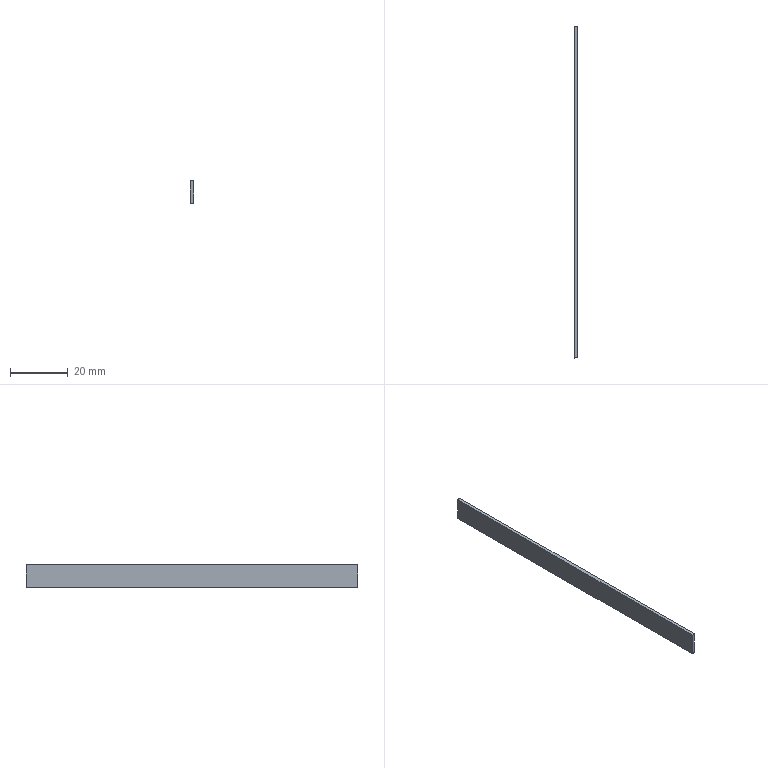Part | SolidWorks | features BaseBody 1 | 1 solid | 6 faces | box 1.056 x 115.104 x 8.015 mm | volume 966.522 mm3 | plane 4 | cylinder 2 | commonest cylinder face diameters 97.2 x1 165.792 x1
STEP:
#1=CARTESIAN_POINT('',(-2128.823,1269.344,-1626.049));
#2=VERTEX_POINT('',#1);
#3=CARTESIAN_POINT('',(-2128.823,1154.24,-1626.049));
#4=VERTEX_POINT('',#3);
#5=CARTESIAN_POINT('',(-2128.823,1269.344,-1626.049));
#6=DIRECTION('',(0.,-1.,0.));
#7=VECTOR('',#6,1000.);
#8=LINE('',#5,#7);
#9=EDGE_CURVE('',#2,#4,#8,.T.);
#10=ORIENTED_EDGE('',*,*,#9,.F.);
#11=CARTESIAN_POINT('',(-2129.879,1269.344,-1626.127));
#12=VERTEX_POINT('',#11);
#13=CARTESIAN_POINT('',(-2132.95,1269.344,-1577.624));
#14=DIRECTION('',(0.,1.,0.));
#15=DIRECTION('',(0.0849,0.,-0.9964));
#16=AXIS2_PLACEMENT_3D('',#13,#14,#15);
#17=CIRCLE('',#16,48.6);
#18=EDGE_CURVE('',#2,#12,#17,.T.);
#19=ORIENTED_EDGE('',*,*,#18,.T.);
#20=CARTESIAN_POINT('',(-2129.879,1154.24,-1626.127));
#21=VERTEX_POINT('',#20);
#22=CARTESIAN_POINT('',(-2129.879,1269.344,-1626.127));
#23=DIRECTION('',(0.,-1.,0.));
#24=VECTOR('',#23,1000.);
#25=LINE('',#22,#24);
#26=EDGE_CURVE('',#12,#21,#25,.T.);
#27=ORIENTED_EDGE('',*,*,#26,.T.);
#28=CARTESIAN_POINT('',(-2132.95,1154.24,-1577.624));
#29=DIRECTION('',(0.,-1.,0.));
#30=DIRECTION('',(0.06317,0.,-0.998));
#31=AXIS2_PLACEMENT_3D('',#28,#29,#30);
#32=CIRCLE('',#31,48.6);
#33=EDGE_CURVE('',#21,#4,#32,.T.);
#34=ORIENTED_EDGE('',*,*,#33,.T.);
#35=EDGE_LOOP('',(#10,#19,#27,#34));
#36=FACE_OUTER_BOUND('',#35,.T.);
#37=CARTESIAN_POINT('',(-2132.95,1275.099,-1577.624));
#38=DIRECTION('',(0.,-1.,0.));
#39=DIRECTION('',(-0.02405,0.,-0.9997));
#40=AXIS2_PLACEMENT_3D('',#37,#38,#39);
#41=CYLINDRICAL_SURFACE('',#40,48.6);
#42=ADVANCED_FACE('',(#36),#41,.F.);
#43=CARTESIAN_POINT('',(-2128.823,1269.344,-1634.018));
#44=VERTEX_POINT('',#43);
#45=CARTESIAN_POINT('',(-2128.823,1154.24,-1634.018));
#46=VERTEX_POINT('',#45);
#47=CARTESIAN_POINT('',(-2128.823,1269.344,-1634.018));
#48=DIRECTION('',(0.,-1.,0.));
#49=VECTOR('',#48,1000.);
#50=LINE('',#47,#49);
#51=EDGE_CURVE('',#44,#46,#50,.T.);
#52=ORIENTED_EDGE('',*,*,#51,.T.);
#53=CARTESIAN_POINT('',(-2129.879,1154.24,-1634.064));
#54=VERTEX_POINT('',#53);
#55=CARTESIAN_POINT('',(-2132.95,1154.24,-1551.224));
#56=DIRECTION('',(0.,-1.,0.));
#57=DIRECTION('',(0.03704,0.,-0.9993));
#58=AXIS2_PLACEMENT_3D('',#55,#56,#57);
#59=CIRCLE('',#58,82.896);
#60=EDGE_CURVE('',#54,#46,#59,.T.);
#61=ORIENTED_EDGE('',*,*,#60,.F.);
#62=CARTESIAN_POINT('',(-2129.879,1269.344,-1634.064));
#63=VERTEX_POINT('',#62);
#64=CARTESIAN_POINT('',(-2129.879,1154.24,-1634.064));
#65=DIRECTION('',(0.,1.,0.));
#66=VECTOR('',#65,1000.);
#67=LINE('',#64,#66);
#68=EDGE_CURVE('',#54,#63,#67,.T.);
#69=ORIENTED_EDGE('',*,*,#68,.T.);
#70=CARTESIAN_POINT('',(-2132.95,1269.344,-1551.224));
#71=DIRECTION('',(0.,1.,0.));
#72=DIRECTION('',(0.04978,0.,-0.9988));
#73=AXIS2_PLACEMENT_3D('',#70,#71,#72);
#74=CIRCLE('',#73,82.896);
#75=EDGE_CURVE('',#44,#63,#74,.T.);
#76=ORIENTED_EDGE('',*,*,#75,.F.);
#77=EDGE_LOOP('',(#52,#61,#69,#76));
#78=FACE_OUTER_BOUND('',#77,.T.);
#79=CARTESIAN_POINT('',(-2132.95,1275.099,-1551.224));
#80=DIRECTION('',(0.,1.,0.));
#81=DIRECTION('',(0.1366,0.,-0.9906));
#82=AXIS2_PLACEMENT_3D('',#79,#80,#81);
#83=CYLINDRICAL_SURFACE('',#82,82.896);
#84=ADVANCED_FACE('',(#78),#83,.T.);
#85=ORIENTED_EDGE('',*,*,#9,.T.);
#86=CARTESIAN_POINT('',(-2128.823,1154.24,-1634.018));
#87=DIRECTION('',(0.000000002,-0.000000002,1.));
#88=VECTOR('',#87,1000.);
#89=LINE('',#86,#88);
#90=EDGE_CURVE('',#46,#4,#89,.T.);
#91=ORIENTED_EDGE('',*,*,#90,.F.);
#92=ORIENTED_EDGE('',*,*,#51,.F.);
#93=CARTESIAN_POINT('',(-2128.823,1269.344,-1626.049));
#94=DIRECTION('',(-0.000000002,-0.000000002,-1.));
#95=VECTOR('',#94,1000.);
#96=LINE('',#93,#95);
#97=EDGE_CURVE('',#2,#44,#96,.T.);
#98=ORIENTED_EDGE('',*,*,#97,.F.);
#99=EDGE_LOOP('',(#85,#91,#92,#98));
#100=FACE_OUTER_BOUND('',#99,.T.);
#101=CARTESIAN_POINT('',(-2128.823,1275.099,-1639.773));
#102=DIRECTION('',(1.,0.,0.));
#103=DIRECTION('',(0.,1.,0.));
#104=AXIS2_PLACEMENT_3D('',#101,#102,#103);
#105=PLANE('',#104);
#106=ADVANCED_FACE('',(#100),#105,.T.);
#107=ORIENTED_EDGE('',*,*,#18,.F.);
#108=ORIENTED_EDGE('',*,*,#97,.T.);
#109=ORIENTED_EDGE('',*,*,#75,.T.);
#110=CARTESIAN_POINT('',(-2129.879,1269.344,-1634.064));
#111=DIRECTION('',(0.,0.000000002,1.));
#112=VECTOR('',#111,1000.);
#113=LINE('',#110,#112);
#114=EDGE_CURVE('',#63,#12,#113,.T.);
#115=ORIENTED_EDGE('',*,*,#114,.T.);
#116=EDGE_LOOP('',(#107,#108,#109,#115));
#117=FACE_OUTER_BOUND('',#116,.T.);
#118=CARTESIAN_POINT('',(-2128.423,1269.344,-1634.464));
#119=DIRECTION('',(0.,1.,0.));
#120=DIRECTION('',(1.,0.,0.));
#121=AXIS2_PLACEMENT_3D('',#118,#119,#120);
#122=PLANE('',#121);
#123=ADVANCED_FACE('',(#117),#122,.T.);
#124=ORIENTED_EDGE('',*,*,#68,.F.);
#125=CARTESIAN_POINT('',(-2129.879,1154.24,-1626.127));
#126=DIRECTION('',(0.,0.,-1.));
#127=VECTOR('',#126,1000.);
#128=LINE('',#125,#127);
#129=EDGE_CURVE('',#21,#54,#128,.T.);
#130=ORIENTED_EDGE('',*,*,#129,.F.);
#131=ORIENTED_EDGE('',*,*,#26,.F.);
#132=ORIENTED_EDGE('',*,*,#114,.F.);
#133=EDGE_LOOP('',(#124,#130,#131,#132));
#134=FACE_OUTER_BOUND('',#133,.T.);
#135=CARTESIAN_POINT('',(-2129.879,1275.099,-1620.372));
#136=DIRECTION('',(-1.,0.,0.));
#137=DIRECTION('',(0.,0.,1.));
#138=AXIS2_PLACEMENT_3D('',#135,#136,#137);
#139=PLANE('',#138);
#140=ADVANCED_FACE('',(#134),#139,.T.);
#141=ORIENTED_EDGE('',*,*,#33,.F.);
#142=ORIENTED_EDGE('',*,*,#129,.T.);
#143=ORIENTED_EDGE('',*,*,#60,.T.);
#144=ORIENTED_EDGE('',*,*,#90,.T.);
#145=EDGE_LOOP('',(#141,#142,#143,#144));
#146=FACE_OUTER_BOUND('',#145,.T.);
#147=CARTESIAN_POINT('',(-2130.28,1154.24,-1634.464));
#148=DIRECTION('',(0.,-1.,0.));
#149=DIRECTION('',(0.,0.,-1.));
#150=AXIS2_PLACEMENT_3D('',#147,#148,#149);
#151=PLANE('',#150);
#152=ADVANCED_FACE('',(#146),#151,.T.);
#153=CLOSED_SHELL('',(#42,#84,#106,#123,#140,#152));
#154=MANIFOLD_SOLID_BREP('',#153);
#155=CARTESIAN_POINT('',(0.,0.,0.));
#156=DIRECTION('',(0.,0.,1.));
#157=DIRECTION('',(1.,0.,0.));
#158=AXIS2_PLACEMENT_3D('',#155,#156,#157);
#159=(LENGTH_UNIT()NAMED_UNIT(*)SI_UNIT(.MILLI.,.METRE.));
#160=UNCERTAINTY_MEASURE_WITH_UNIT(LENGTH_MEASURE(0.00001),#159,'','');
#161=(NAMED_UNIT(*)PLANE_ANGLE_UNIT()SI_UNIT($,.RADIAN.));
#162=(NAMED_UNIT(*)SI_UNIT($,.STERADIAN.)SOLID_ANGLE_UNIT());
#163=(GEOMETRIC_REPRESENTATION_CONTEXT(3)GLOBAL_UNCERTAINTY_ASSIGNED_CONTEXT((#160))GLOBAL_UNIT_ASSIGNED_CONTEXT((#159,#161,#162))REPRESENTATION_CONTEXT('',''));
#164=ADVANCED_BREP_SHAPE_REPRESENTATION('',(#154,#158),#163);